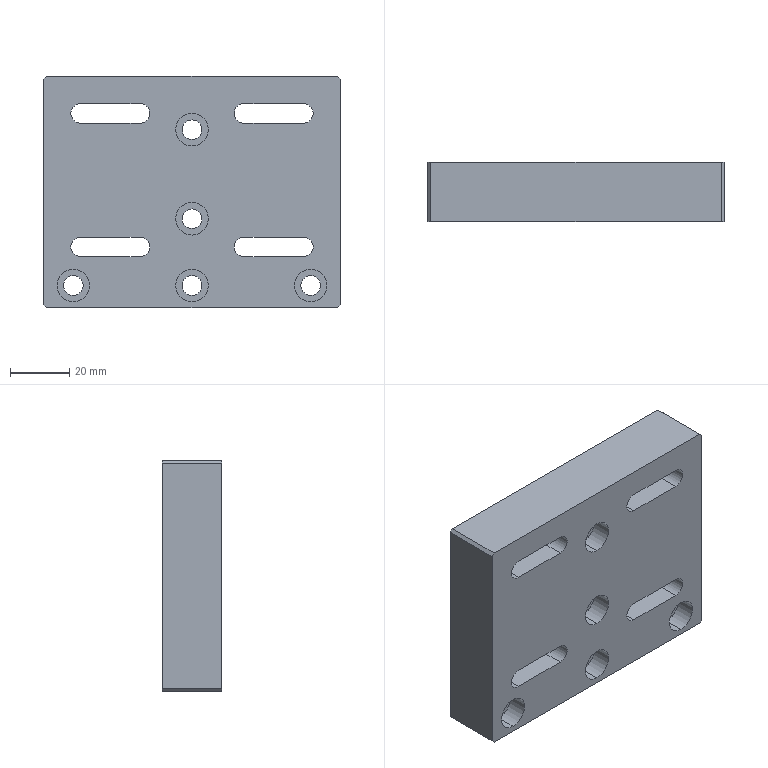Part | SolidWorks | features BaseBody 1 | 1 solid | 71 faces | box 100 x 20 x 78 mm | volume 133126 mm3 | cylinder 36 | plane 35 | commonest cylinder face diameters 6.6 x18 11 x18